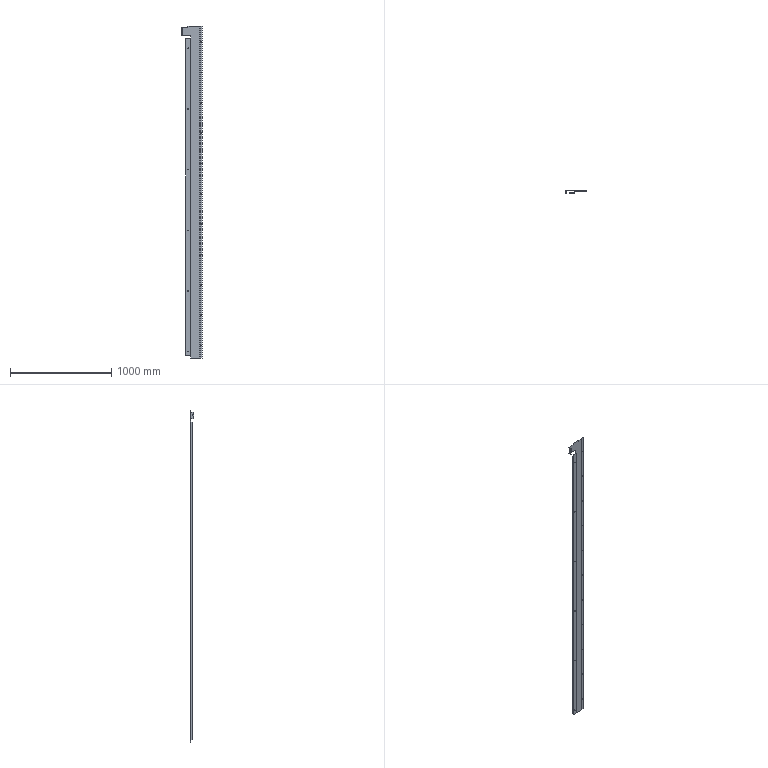Part | STEP file | TS-S96 | 1 solid | 101 faces | box 199 x 33 x 3283 mm | volume 719864 mm3 | cylinder 54 | plane 47 | commonest cylinder face diameters 5.4 x36 0.4 x5 2.8 x5 10 x5 30 x2 20 x1